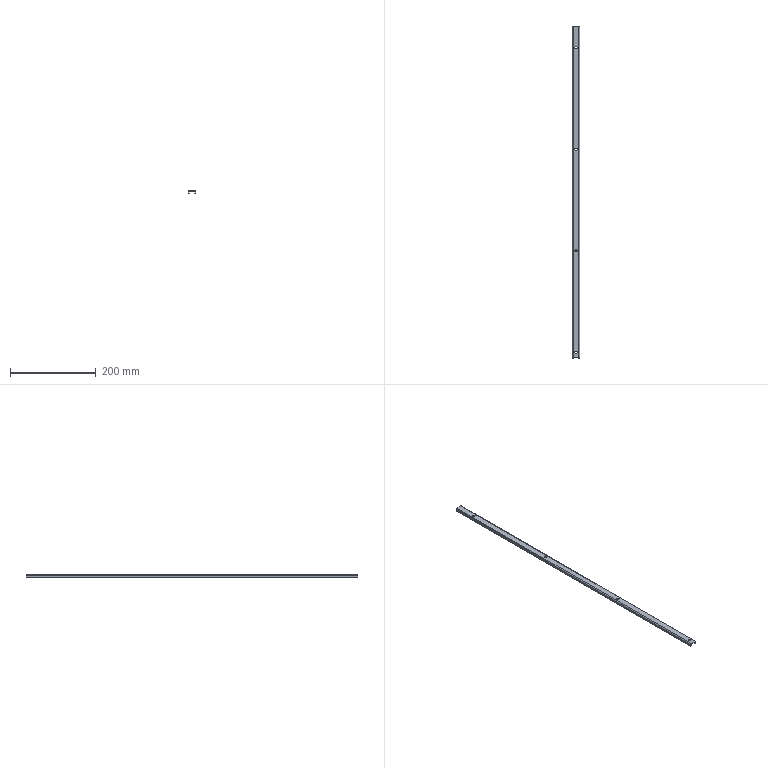Part | NX | features BREP 1 | 1 solid | 40 faces | box 17 x 774.5 x 7 mm | volume 39998 mm3 | plane 22 | cone 8 | cylinder 6 | torus 4 | commonest cylinder face diameters 0.2 x2 2 x2 4.2 x2
STEP:
#1=CARTESIAN_POINT('',(-2.7,336.75,2.));
#2=VERTEX_POINT('',#1);
#3=CARTESIAN_POINT('',(2.7,336.75,2.));
#4=VERTEX_POINT('',#3);
#5=CARTESIAN_POINT('',(0.,336.75,2.));
#6=DIRECTION('',(0.,0.,1.));
#7=DIRECTION('',(1.,0.,0.));
#8=AXIS2_PLACEMENT_3D('',#5,#6,#7);
#9=CIRCLE('',#8,2.7);
#10=EDGE_CURVE('',#2,#4,#9,.T.);
#11=ORIENTED_EDGE('',*,*,#10,.T.);
#12=CARTESIAN_POINT('',(4.7,336.75,0.));
#13=VERTEX_POINT('',#12);
#14=CARTESIAN_POINT('',(4.7,336.75,0.));
#15=DIRECTION('',(0.7071,0.,-0.7071));
#16=VECTOR('',#15,1000.);
#17=LINE('',#14,#16);
#18=EDGE_CURVE('',#4,#13,#17,.T.);
#19=ORIENTED_EDGE('',*,*,#18,.T.);
#20=CARTESIAN_POINT('',(-4.7,336.75,0.));
#21=VERTEX_POINT('',#20);
#22=CARTESIAN_POINT('',(0.,336.75,0.));
#23=DIRECTION('',(0.,0.,-1.));
#24=DIRECTION('',(-1.,0.,0.));
#25=AXIS2_PLACEMENT_3D('',#22,#23,#24);
#26=CIRCLE('',#25,4.7);
#27=EDGE_CURVE('',#13,#21,#26,.T.);
#28=ORIENTED_EDGE('',*,*,#27,.T.);
#29=CARTESIAN_POINT('',(-4.7,336.75,0.));
#30=DIRECTION('',(-0.7071,0.,-0.7071));
#31=VECTOR('',#30,1000.);
#32=LINE('',#29,#31);
#33=EDGE_CURVE('',#2,#21,#32,.T.);
#34=ORIENTED_EDGE('',*,*,#33,.F.);
#35=EDGE_LOOP('',(#11,#19,#28,#34));
#36=FACE_BOUND('',#35,.T.);
#37=CARTESIAN_POINT('',(0.,336.75,0.));
#38=DIRECTION('',(0.,0.,-1.));
#39=DIRECTION('',(-1.,0.,0.));
#40=AXIS2_PLACEMENT_3D('',#37,#38,#39);
#41=CONICAL_SURFACE('',#40,4.7,0.7854);
#42=ADVANCED_FACE('',(#36),#41,.F.);
#43=CARTESIAN_POINT('',(-2.7,99.75,2.));
#44=VERTEX_POINT('',#43);
#45=CARTESIAN_POINT('',(2.7,99.75,2.));
#46=VERTEX_POINT('',#45);
#47=CARTESIAN_POINT('',(0.,99.75,2.));
#48=DIRECTION('',(0.,0.,1.));
#49=DIRECTION('',(1.,0.,0.));
#50=AXIS2_PLACEMENT_3D('',#47,#48,#49);
#51=CIRCLE('',#50,2.7);
#52=EDGE_CURVE('',#44,#46,#51,.T.);
#53=ORIENTED_EDGE('',*,*,#52,.T.);
#54=CARTESIAN_POINT('',(4.7,99.75,0.));
#55=VERTEX_POINT('',#54);
#56=CARTESIAN_POINT('',(4.7,99.75,0.));
#57=DIRECTION('',(0.7071,0.,-0.7071));
#58=VECTOR('',#57,1000.);
#59=LINE('',#56,#58);
#60=EDGE_CURVE('',#46,#55,#59,.T.);
#61=ORIENTED_EDGE('',*,*,#60,.T.);
#62=CARTESIAN_POINT('',(-4.7,99.75,0.));
#63=VERTEX_POINT('',#62);
#64=CARTESIAN_POINT('',(0.,99.75,0.));
#65=DIRECTION('',(0.,0.,-1.));
#66=DIRECTION('',(-1.,0.,0.));
#67=AXIS2_PLACEMENT_3D('',#64,#65,#66);
#68=CIRCLE('',#67,4.7);
#69=EDGE_CURVE('',#55,#63,#68,.T.);
#70=ORIENTED_EDGE('',*,*,#69,.T.);
#71=CARTESIAN_POINT('',(-4.7,99.75,0.));
#72=DIRECTION('',(-0.7071,0.,-0.7071));
#73=VECTOR('',#72,1000.);
#74=LINE('',#71,#73);
#75=EDGE_CURVE('',#44,#63,#74,.T.);
#76=ORIENTED_EDGE('',*,*,#75,.F.);
#77=EDGE_LOOP('',(#53,#61,#70,#76));
#78=FACE_BOUND('',#77,.T.);
#79=CARTESIAN_POINT('',(0.,99.75,0.));
#80=DIRECTION('',(0.,0.,-1.));
#81=DIRECTION('',(-1.,0.,0.));
#82=AXIS2_PLACEMENT_3D('',#79,#80,#81);
#83=CONICAL_SURFACE('',#82,4.7,0.7854);
#84=ADVANCED_FACE('',(#78),#83,.F.);
#85=CARTESIAN_POINT('',(-2.7,-137.25,2.));
#86=VERTEX_POINT('',#85);
#87=CARTESIAN_POINT('',(2.7,-137.25,2.));
#88=VERTEX_POINT('',#87);
#89=CARTESIAN_POINT('',(0.,-137.25,2.));
#90=DIRECTION('',(0.,0.,1.));
#91=DIRECTION('',(1.,0.,0.));
#92=AXIS2_PLACEMENT_3D('',#89,#90,#91);
#93=CIRCLE('',#92,2.7);
#94=EDGE_CURVE('',#86,#88,#93,.T.);
#95=ORIENTED_EDGE('',*,*,#94,.T.);
#96=CARTESIAN_POINT('',(4.7,-137.25,0.));
#97=VERTEX_POINT('',#96);
#98=CARTESIAN_POINT('',(4.7,-137.25,0.));
#99=DIRECTION('',(0.7071,0.,-0.7071));
#100=VECTOR('',#99,1000.);
#101=LINE('',#98,#100);
#102=EDGE_CURVE('',#88,#97,#101,.T.);
#103=ORIENTED_EDGE('',*,*,#102,.T.);
#104=CARTESIAN_POINT('',(-4.7,-137.25,0.));
#105=VERTEX_POINT('',#104);
#106=CARTESIAN_POINT('',(0.,-137.25,0.));
#107=DIRECTION('',(0.,0.,-1.));
#108=DIRECTION('',(-1.,0.,0.));
#109=AXIS2_PLACEMENT_3D('',#106,#107,#108);
#110=CIRCLE('',#109,4.7);
#111=EDGE_CURVE('',#97,#105,#110,.T.);
#112=ORIENTED_EDGE('',*,*,#111,.T.);
#113=CARTESIAN_POINT('',(-4.7,-137.25,0.));
#114=DIRECTION('',(-0.7071,0.,-0.7071));
#115=VECTOR('',#114,1000.);
#116=LINE('',#113,#115);
#117=EDGE_CURVE('',#86,#105,#116,.T.);
#118=ORIENTED_EDGE('',*,*,#117,.F.);
#119=EDGE_LOOP('',(#95,#103,#112,#118));
#120=FACE_BOUND('',#119,.T.);
#121=CARTESIAN_POINT('',(0.,-137.25,0.));
#122=DIRECTION('',(0.,0.,-1.));
#123=DIRECTION('',(-1.,0.,0.));
#124=AXIS2_PLACEMENT_3D('',#121,#122,#123);
#125=CONICAL_SURFACE('',#124,4.7,0.7854);
#126=ADVANCED_FACE('',(#120),#125,.F.);
#127=CARTESIAN_POINT('',(-2.7,-374.25,2.));
#128=VERTEX_POINT('',#127);
#129=CARTESIAN_POINT('',(2.7,-374.25,2.));
#130=VERTEX_POINT('',#129);
#131=CARTESIAN_POINT('',(0.,-374.25,2.));
#132=DIRECTION('',(0.,0.,1.));
#133=DIRECTION('',(1.,0.,0.));
#134=AXIS2_PLACEMENT_3D('',#131,#132,#133);
#135=CIRCLE('',#134,2.7);
#136=EDGE_CURVE('',#128,#130,#135,.T.);
#137=ORIENTED_EDGE('',*,*,#136,.T.);
#138=CARTESIAN_POINT('',(4.7,-374.25,0.));
#139=VERTEX_POINT('',#138);
#140=CARTESIAN_POINT('',(4.7,-374.25,0.));
#141=DIRECTION('',(0.7071,0.,-0.7071));
#142=VECTOR('',#141,1000.);
#143=LINE('',#140,#142);
#144=EDGE_CURVE('',#130,#139,#143,.T.);
#145=ORIENTED_EDGE('',*,*,#144,.T.);
#146=CARTESIAN_POINT('',(-4.7,-374.25,0.));
#147=VERTEX_POINT('',#146);
#148=CARTESIAN_POINT('',(0.,-374.25,0.));
#149=DIRECTION('',(0.,0.,-1.));
#150=DIRECTION('',(-1.,0.,0.));
#151=AXIS2_PLACEMENT_3D('',#148,#149,#150);
#152=CIRCLE('',#151,4.7);
#153=EDGE_CURVE('',#139,#147,#152,.T.);
#154=ORIENTED_EDGE('',*,*,#153,.T.);
#155=CARTESIAN_POINT('',(-4.7,-374.25,0.));
#156=DIRECTION('',(-0.7071,0.,-0.7071));
#157=VECTOR('',#156,1000.);
#158=LINE('',#155,#157);
#159=EDGE_CURVE('',#128,#147,#158,.T.);
#160=ORIENTED_EDGE('',*,*,#159,.F.);
#161=EDGE_LOOP('',(#137,#145,#154,#160));
#162=FACE_BOUND('',#161,.T.);
#163=CARTESIAN_POINT('',(0.,-374.25,0.));
#164=DIRECTION('',(0.,0.,-1.));
#165=DIRECTION('',(-1.,0.,0.));
#166=AXIS2_PLACEMENT_3D('',#163,#164,#165);
#167=CONICAL_SURFACE('',#166,4.7,0.7854);
#168=ADVANCED_FACE('',(#162),#167,.F.);
#169=CARTESIAN_POINT('',(-6.4,386.25,0.));
#170=VERTEX_POINT('',#169);
#171=CARTESIAN_POINT('',(-6.4,-386.25,0.));
#172=VERTEX_POINT('',#171);
#173=CARTESIAN_POINT('',(-6.4,387.25,0.));
#174=DIRECTION('',(0.,-1.,0.));
#175=VECTOR('',#174,1000.);
#176=LINE('',#173,#175);
#177=EDGE_CURVE('',#170,#172,#176,.T.);
#178=ORIENTED_EDGE('',*,*,#177,.F.);
#179=CARTESIAN_POINT('',(6.4,386.25,0.));
#180=VERTEX_POINT('',#179);
#181=CARTESIAN_POINT('',(6.4,386.25,0.));
#182=DIRECTION('',(1.,0.,0.));
#183=VECTOR('',#182,1000.);
#184=LINE('',#181,#183);
#185=EDGE_CURVE('',#170,#180,#184,.T.);
#186=ORIENTED_EDGE('',*,*,#185,.T.);
#187=CARTESIAN_POINT('',(6.4,-386.25,0.));
#188=VERTEX_POINT('',#187);
#189=CARTESIAN_POINT('',(6.4,387.25,0.));
#190=DIRECTION('',(0.,-1.,0.));
#191=VECTOR('',#190,1000.);
#192=LINE('',#189,#191);
#193=EDGE_CURVE('',#180,#188,#192,.T.);
#194=ORIENTED_EDGE('',*,*,#193,.T.);
#195=CARTESIAN_POINT('',(-6.4,-386.25,0.));
#196=DIRECTION('',(-1.,0.,0.));
#197=VECTOR('',#196,1000.);
#198=LINE('',#195,#197);
#199=EDGE_CURVE('',#188,#172,#198,.T.);
#200=ORIENTED_EDGE('',*,*,#199,.T.);
#201=EDGE_LOOP('',(#178,#186,#194,#200));
#202=FACE_BOUND('',#201,.T.);
#203=CARTESIAN_POINT('',(0.,336.75,0.));
#204=DIRECTION('',(0.,0.,-1.));
#205=DIRECTION('',(-1.,0.,0.));
#206=AXIS2_PLACEMENT_3D('',#203,#204,#205);
#207=CIRCLE('',#206,4.7);
#208=EDGE_CURVE('',#21,#13,#207,.T.);
#209=ORIENTED_EDGE('',*,*,#208,.F.);
#210=ORIENTED_EDGE('',*,*,#27,.F.);
#211=EDGE_LOOP('',(#209,#210));
#212=FACE_BOUND('',#211,.T.);
#213=CARTESIAN_POINT('',(0.,99.75,0.));
#214=DIRECTION('',(0.,0.,-1.));
#215=DIRECTION('',(-1.,0.,0.));
#216=AXIS2_PLACEMENT_3D('',#213,#214,#215);
#217=CIRCLE('',#216,4.7);
#218=EDGE_CURVE('',#63,#55,#217,.T.);
#219=ORIENTED_EDGE('',*,*,#218,.F.);
#220=ORIENTED_EDGE('',*,*,#69,.F.);
#221=EDGE_LOOP('',(#219,#220));
#222=FACE_BOUND('',#221,.T.);
#223=CARTESIAN_POINT('',(0.,-374.25,0.));
#224=DIRECTION('',(0.,0.,-1.));
#225=DIRECTION('',(-1.,0.,0.));
#226=AXIS2_PLACEMENT_3D('',#223,#224,#225);
#227=CIRCLE('',#226,4.7);
#228=EDGE_CURVE('',#147,#139,#227,.T.);
#229=ORIENTED_EDGE('',*,*,#228,.F.);
#230=ORIENTED_EDGE('',*,*,#153,.F.);
#231=EDGE_LOOP('',(#229,#230));
#232=FACE_BOUND('',#231,.T.);
#233=CARTESIAN_POINT('',(0.,-137.25,0.));
#234=DIRECTION('',(0.,0.,-1.));
#235=DIRECTION('',(-1.,0.,0.));
#236=AXIS2_PLACEMENT_3D('',#233,#234,#235);
#237=CIRCLE('',#236,4.7);
#238=EDGE_CURVE('',#105,#97,#237,.T.);
#239=ORIENTED_EDGE('',*,*,#238,.F.);
#240=ORIENTED_EDGE('',*,*,#111,.F.);
#241=EDGE_LOOP('',(#239,#240));
#242=FACE_BOUND('',#241,.T.);
#243=CARTESIAN_POINT('',(-6.5,387.25,0.));
#244=DIRECTION('',(0.,0.,1.));
#245=DIRECTION('',(1.,0.,0.));
#246=AXIS2_PLACEMENT_3D('',#243,#244,#245);
#247=PLANE('',#246);
#248=ADVANCED_FACE('',(#202,#212,#222,#232,#242),#247,.F.);
#249=CARTESIAN_POINT('',(6.4,-387.25,2.));
#250=VERTEX_POINT('',#249);
#251=CARTESIAN_POINT('',(-6.4,-387.25,2.));
#252=VERTEX_POINT('',#251);
#253=CARTESIAN_POINT('',(-6.5,-387.25,2.));
#254=DIRECTION('',(-1.,0.,0.));
#255=VECTOR('',#254,1000.);
#256=LINE('',#253,#255);
#257=EDGE_CURVE('',#250,#252,#256,.T.);
#258=ORIENTED_EDGE('',*,*,#257,.F.);
#259=CARTESIAN_POINT('',(6.4,387.25,2.));
#260=VERTEX_POINT('',#259);
#261=CARTESIAN_POINT('',(6.4,387.25,2.));
#262=DIRECTION('',(0.,-1.,0.));
#263=VECTOR('',#262,1000.);
#264=LINE('',#261,#263);
#265=EDGE_CURVE('',#260,#250,#264,.T.);
#266=ORIENTED_EDGE('',*,*,#265,.F.);
#267=CARTESIAN_POINT('',(-6.4,387.25,2.));
#268=VERTEX_POINT('',#267);
#269=CARTESIAN_POINT('',(-6.5,387.25,2.));
#270=DIRECTION('',(-1.,0.,0.));
#271=VECTOR('',#270,1000.);
#272=LINE('',#269,#271);
#273=EDGE_CURVE('',#260,#268,#272,.T.);
#274=ORIENTED_EDGE('',*,*,#273,.T.);
#275=CARTESIAN_POINT('',(-6.4,387.25,2.));
#276=DIRECTION('',(0.,-1.,0.));
#277=VECTOR('',#276,1000.);
#278=LINE('',#275,#277);
#279=EDGE_CURVE('',#268,#252,#278,.T.);
#280=ORIENTED_EDGE('',*,*,#279,.T.);
#281=EDGE_LOOP('',(#258,#266,#274,#280));
#282=FACE_BOUND('',#281,.T.);
#283=ORIENTED_EDGE('',*,*,#10,.F.);
#284=CARTESIAN_POINT('',(0.,336.75,2.));
#285=DIRECTION('',(0.,0.,1.));
#286=DIRECTION('',(1.,0.,0.));
#287=AXIS2_PLACEMENT_3D('',#284,#285,#286);
#288=CIRCLE('',#287,2.7);
#289=EDGE_CURVE('',#4,#2,#288,.T.);
#290=ORIENTED_EDGE('',*,*,#289,.F.);
#291=EDGE_LOOP('',(#283,#290));
#292=FACE_BOUND('',#291,.T.);
#293=ORIENTED_EDGE('',*,*,#52,.F.);
#294=CARTESIAN_POINT('',(0.,99.75,2.));
#295=DIRECTION('',(0.,0.,1.));
#296=DIRECTION('',(1.,0.,0.));
#297=AXIS2_PLACEMENT_3D('',#294,#295,#296);
#298=CIRCLE('',#297,2.7);
#299=EDGE_CURVE('',#46,#44,#298,.T.);
#300=ORIENTED_EDGE('',*,*,#299,.F.);
#301=EDGE_LOOP('',(#293,#300));
#302=FACE_BOUND('',#301,.T.);
#303=ORIENTED_EDGE('',*,*,#94,.F.);
#304=CARTESIAN_POINT('',(0.,-137.25,2.));
#305=DIRECTION('',(0.,0.,1.));
#306=DIRECTION('',(1.,0.,0.));
#307=AXIS2_PLACEMENT_3D('',#304,#305,#306);
#308=CIRCLE('',#307,2.7);
#309=EDGE_CURVE('',#88,#86,#308,.T.);
#310=ORIENTED_EDGE('',*,*,#309,.F.);
#311=EDGE_LOOP('',(#303,#310));
#312=FACE_BOUND('',#311,.T.);
#313=ORIENTED_EDGE('',*,*,#136,.F.);
#314=CARTESIAN_POINT('',(0.,-374.25,2.));
#315=DIRECTION('',(0.,0.,1.));
#316=DIRECTION('',(1.,0.,0.));
#317=AXIS2_PLACEMENT_3D('',#314,#315,#316);
#318=CIRCLE('',#317,2.7);
#319=EDGE_CURVE('',#130,#128,#318,.T.);
#320=ORIENTED_EDGE('',*,*,#319,.F.);
#321=EDGE_LOOP('',(#313,#320));
#322=FACE_BOUND('',#321,.T.);
#323=CARTESIAN_POINT('',(-6.5,387.25,2.));
#324=DIRECTION('',(0.,0.,1.));
#325=DIRECTION('',(1.,0.,0.));
#326=AXIS2_PLACEMENT_3D('',#323,#324,#325);
#327=PLANE('',#326);
#328=ADVANCED_FACE('',(#282,#292,#302,#312,#322),#327,.T.);
#329=CARTESIAN_POINT('',(7.5,387.25,-0.1));
#330=VERTEX_POINT('',#329);
#331=CARTESIAN_POINT('',(8.5,387.25,-0.1));
#332=VERTEX_POINT('',#331);
#333=CARTESIAN_POINT('',(6.5,387.25,-0.1));
#334=DIRECTION('',(1.,0.,0.));
#335=VECTOR('',#334,1000.);
#336=LINE('',#333,#335);
#337=EDGE_CURVE('',#330,#332,#336,.T.);
#338=ORIENTED_EDGE('',*,*,#337,.F.);
#339=CARTESIAN_POINT('',(6.4,387.25,1.));
#340=VERTEX_POINT('',#339);
#341=CARTESIAN_POINT('',(6.4,387.25,-0.1));
#342=DIRECTION('',(0.,-1.,0.));
#343=DIRECTION('',(0.,0.,1.));
#344=AXIS2_PLACEMENT_3D('',#341,#342,#343);
#345=CIRCLE('',#344,1.1);
#346=EDGE_CURVE('',#330,#340,#345,.T.);
#347=ORIENTED_EDGE('',*,*,#346,.T.);
#348=CARTESIAN_POINT('',(6.4,387.25,2.));
#349=DIRECTION('',(0.,0.,-1.));
#350=VECTOR('',#349,1000.);
#351=LINE('',#348,#350);
#352=EDGE_CURVE('',#260,#340,#351,.T.);
#353=ORIENTED_EDGE('',*,*,#352,.F.);
#354=CARTESIAN_POINT('',(6.4,387.25,-0.1));
#355=DIRECTION('',(0.,-1.,0.));
#356=DIRECTION('',(1.,0.,0.));
#357=AXIS2_PLACEMENT_3D('',#354,#355,#356);
#358=CIRCLE('',#357,2.1);
#359=EDGE_CURVE('',#332,#260,#358,.T.);
#360=ORIENTED_EDGE('',*,*,#359,.F.);
#361=EDGE_LOOP('',(#338,#347,#353,#360));
#362=FACE_BOUND('',#361,.T.);
#363=CARTESIAN_POINT('',(6.5,387.25,-0.1));
#364=DIRECTION('',(0.,1.,0.));
#365=DIRECTION('',(1.,0.,0.));
#366=AXIS2_PLACEMENT_3D('',#363,#364,#365);
#367=PLANE('',#366);
#368=ADVANCED_FACE('',(#362),#367,.T.);
#369=CARTESIAN_POINT('',(8.5,387.25,-4.));
#370=VERTEX_POINT('',#369);
#371=CARTESIAN_POINT('',(8.5,387.25,0.));
#372=DIRECTION('',(0.,0.,1.));
#373=VECTOR('',#372,1000.);
#374=LINE('',#371,#373);
#375=EDGE_CURVE('',#370,#332,#374,.T.);
#376=ORIENTED_EDGE('',*,*,#375,.F.);
#377=CARTESIAN_POINT('',(6.5,387.25,-4.));
#378=VERTEX_POINT('',#377);
#379=CARTESIAN_POINT('',(6.4,387.25,-4.));
#380=DIRECTION('',(-1.,0.,0.));
#381=VECTOR('',#380,1000.);
#382=LINE('',#379,#381);
#383=EDGE_CURVE('',#370,#378,#382,.T.);
#384=ORIENTED_EDGE('',*,*,#383,.T.);
#385=CARTESIAN_POINT('',(6.5,387.25,-1.195));
#386=VERTEX_POINT('',#385);
#387=CARTESIAN_POINT('',(6.5,387.25,0.));
#388=DIRECTION('',(0.,0.,1.));
#389=VECTOR('',#388,1000.);
#390=LINE('',#387,#389);
#391=EDGE_CURVE('',#378,#386,#390,.T.);
#392=ORIENTED_EDGE('',*,*,#391,.T.);
#393=CARTESIAN_POINT('',(6.4,387.25,-0.1));
#394=DIRECTION('',(0.,-1.,0.));
#395=DIRECTION('',(0.,0.,1.));
#396=AXIS2_PLACEMENT_3D('',#393,#394,#395);
#397=CIRCLE('',#396,1.1);
#398=EDGE_CURVE('',#386,#330,#397,.T.);
#399=ORIENTED_EDGE('',*,*,#398,.T.);
#400=ORIENTED_EDGE('',*,*,#337,.T.);
#401=EDGE_LOOP('',(#376,#384,#392,#399,#400));
#402=FACE_BOUND('',#401,.T.);
#403=CARTESIAN_POINT('',(6.4,387.25,2.));
#404=DIRECTION('',(0.,1.,0.));
#405=DIRECTION('',(1.,0.,0.));
#406=AXIS2_PLACEMENT_3D('',#403,#404,#405);
#407=PLANE('',#406);
#408=ADVANCED_FACE('',(#402),#407,.T.);
#409=CARTESIAN_POINT('',(6.4,-387.25,1.));
#410=VERTEX_POINT('',#409);
#411=CARTESIAN_POINT('',(6.4,-387.25,0.));
#412=DIRECTION('',(0.,0.,1.));
#413=VECTOR('',#412,1000.);
#414=LINE('',#411,#413);
#415=EDGE_CURVE('',#410,#250,#414,.T.);
#416=ORIENTED_EDGE('',*,*,#415,.F.);
#417=CARTESIAN_POINT('',(7.5,-387.25,-0.1));
#418=VERTEX_POINT('',#417);
#419=CARTESIAN_POINT('',(6.4,-387.25,-0.1));
#420=DIRECTION('',(0.,1.,0.));
#421=DIRECTION('',(0.,0.,-1.));
#422=AXIS2_PLACEMENT_3D('',#419,#420,#421);
#423=CIRCLE('',#422,1.1);
#424=EDGE_CURVE('',#410,#418,#423,.T.);
#425=ORIENTED_EDGE('',*,*,#424,.T.);
#426=CARTESIAN_POINT('',(8.5,-387.25,-0.1));
#427=VERTEX_POINT('',#426);
#428=CARTESIAN_POINT('',(8.5,-387.25,-0.1));
#429=DIRECTION('',(-1.,0.,0.));
#430=VECTOR('',#429,1000.);
#431=LINE('',#428,#430);
#432=EDGE_CURVE('',#427,#418,#431,.T.);
#433=ORIENTED_EDGE('',*,*,#432,.F.);
#434=CARTESIAN_POINT('',(6.4,-387.25,-0.1));
#435=DIRECTION('',(0.,-1.,0.));
#436=DIRECTION('',(1.,0.,0.));
#437=AXIS2_PLACEMENT_3D('',#434,#435,#436);
#438=CIRCLE('',#437,2.1);
#439=EDGE_CURVE('',#427,#250,#438,.T.);
#440=ORIENTED_EDGE('',*,*,#439,.T.);
#441=EDGE_LOOP('',(#416,#425,#433,#440));
#442=FACE_BOUND('',#441,.T.);
#443=CARTESIAN_POINT('',(6.4,-387.25,0.));
#444=DIRECTION('',(0.,-1.,0.));
#445=DIRECTION('',(0.,0.,-1.));
#446=AXIS2_PLACEMENT_3D('',#443,#444,#445);
#447=PLANE('',#446);
#448=ADVANCED_FACE('',(#442),#447,.T.);
#449=CARTESIAN_POINT('',(-6.4,-387.25,1.));
#450=VERTEX_POINT('',#449);
#451=CARTESIAN_POINT('',(-6.4,-387.25,2.));
#452=DIRECTION('',(0.,0.,-1.));
#453=VECTOR('',#452,1000.);
#454=LINE('',#451,#453);
#455=EDGE_CURVE('',#252,#450,#454,.T.);
#456=ORIENTED_EDGE('',*,*,#455,.T.);
#457=CARTESIAN_POINT('',(6.4,-387.25,1.));
#458=DIRECTION('',(1.,0.,0.));
#459=VECTOR('',#458,1000.);
#460=LINE('',#457,#459);
#461=EDGE_CURVE('',#450,#410,#460,.T.);
#462=ORIENTED_EDGE('',*,*,#461,.T.);
#463=ORIENTED_EDGE('',*,*,#415,.T.);
#464=ORIENTED_EDGE('',*,*,#257,.T.);
#465=EDGE_LOOP('',(#456,#462,#463,#464));
#466=FACE_BOUND('',#465,.T.);
#467=CARTESIAN_POINT('',(8.5,-387.25,-0.1));
#468=DIRECTION('',(0.,-1.,0.));
#469=DIRECTION('',(0.,0.,-1.));
#470=AXIS2_PLACEMENT_3D('',#467,#468,#469);
#471=PLANE('',#470);
#472=ADVANCED_FACE('',(#466),#471,.T.);
#473=CARTESIAN_POINT('',(-6.4,387.25,1.));
#474=VERTEX_POINT('',#473);
#475=CARTESIAN_POINT('',(-6.4,387.25,0.));
#476=DIRECTION('',(0.,0.,1.));
#477=VECTOR('',#476,1000.);
#478=LINE('',#475,#477);
#479=EDGE_CURVE('',#474,#268,#478,.T.);
#480=ORIENTED_EDGE('',*,*,#479,.F.);
#481=CARTESIAN_POINT('',(-7.5,387.25,-0.1));
#482=VERTEX_POINT('',#481);
#483=CARTESIAN_POINT('',(-6.4,387.25,-0.1));
#484=DIRECTION('',(0.,-1.,0.));
#485=DIRECTION('',(0.,0.,1.));
#486=AXIS2_PLACEMENT_3D('',#483,#484,#485);
#487=CIRCLE('',#486,1.1);
#488=EDGE_CURVE('',#474,#482,#487,.T.);
#489=ORIENTED_EDGE('',*,*,#488,.T.);
#490=CARTESIAN_POINT('',(-8.5,387.25,-0.1));
#491=VERTEX_POINT('',#490);
#492=CARTESIAN_POINT('',(-8.5,387.25,-0.1));
#493=DIRECTION('',(1.,0.,0.));
#494=VECTOR('',#493,1000.);
#495=LINE('',#492,#494);
#496=EDGE_CURVE('',#491,#482,#495,.T.);
#497=ORIENTED_EDGE('',*,*,#496,.F.);
#498=CARTESIAN_POINT('',(-6.4,387.25,-0.1));
#499=DIRECTION('',(0.,-1.,0.));
#500=DIRECTION('',(1.,0.,0.));
#501=AXIS2_PLACEMENT_3D('',#498,#499,#500);
#502=CIRCLE('',#501,2.1);
#503=EDGE_CURVE('',#268,#491,#502,.T.);
#504=ORIENTED_EDGE('',*,*,#503,.F.);
#505=EDGE_LOOP('',(#480,#489,#497,#504));
#506=FACE_BOUND('',#505,.T.);
#507=CARTESIAN_POINT('',(-6.4,387.25,0.));
#508=DIRECTION('',(0.,1.,0.));
#509=DIRECTION('',(1.,0.,0.));
#510=AXIS2_PLACEMENT_3D('',#507,#508,#509);
#511=PLANE('',#510);
#512=ADVANCED_FACE('',(#506),#511,.T.);
#513=ORIENTED_EDGE('',*,*,#352,.T.);
#514=CARTESIAN_POINT('',(-6.4,387.25,1.));
#515=DIRECTION('',(-1.,0.,0.));
#516=VECTOR('',#515,1000.);
#517=LINE('',#514,#516);
#518=EDGE_CURVE('',#340,#474,#517,.T.);
#519=ORIENTED_EDGE('',*,*,#518,.T.);
#520=ORIENTED_EDGE('',*,*,#479,.T.);
#521=ORIENTED_EDGE('',*,*,#273,.F.);
#522=EDGE_LOOP('',(#513,#519,#520,#521));
#523=FACE_BOUND('',#522,.T.);
#524=CARTESIAN_POINT('',(-8.5,387.25,-0.1));
#525=DIRECTION('',(0.,1.,0.));
#526=DIRECTION('',(1.,0.,0.));
#527=AXIS2_PLACEMENT_3D('',#524,#525,#526);
#528=PLANE('',#527);
#529=ADVANCED_FACE('',(#523),#528,.T.);
#530=CARTESIAN_POINT('',(-7.5,-387.25,-0.1));
#531=VERTEX_POINT('',#530);
#532=CARTESIAN_POINT('',(-8.5,-387.25,-0.1));
#533=VERTEX_POINT('',#532);
#534=CARTESIAN_POINT('',(-6.5,-387.25,-0.1));
#535=DIRECTION('',(-1.,0.,0.));
#536=VECTOR('',#535,1000.);
#537=LINE('',#534,#536);
#538=EDGE_CURVE('',#531,#533,#537,.T.);
#539=ORIENTED_EDGE('',*,*,#538,.F.);
#540=CARTESIAN_POINT('',(-6.4,-387.25,-0.1));
#541=DIRECTION('',(0.,1.,0.));
#542=DIRECTION('',(0.,0.,-1.));
#543=AXIS2_PLACEMENT_3D('',#540,#541,#542);
#544=CIRCLE('',#543,1.1);
#545=EDGE_CURVE('',#531,#450,#544,.T.);
#546=ORIENTED_EDGE('',*,*,#545,.T.);
#547=ORIENTED_EDGE('',*,*,#455,.F.);
#548=CARTESIAN_POINT('',(-6.4,-387.25,-0.1));
#549=DIRECTION('',(0.,-1.,0.));
#550=DIRECTION('',(1.,0.,0.));
#551=AXIS2_PLACEMENT_3D('',#548,#549,#550);
#552=CIRCLE('',#551,2.1);
#553=EDGE_CURVE('',#252,#533,#552,.T.);
#554=ORIENTED_EDGE('',*,*,#553,.T.);
#555=EDGE_LOOP('',(#539,#546,#547,#554));
#556=FACE_BOUND('',#555,.T.);
#557=CARTESIAN_POINT('',(-6.5,-387.25,-0.1));
#558=DIRECTION('',(0.,-1.,0.));
#559=DIRECTION('',(0.,0.,-1.));
#560=AXIS2_PLACEMENT_3D('',#557,#558,#559);
#561=PLANE('',#560);
#562=ADVANCED_FACE('',(#556),#561,.T.);
#563=CARTESIAN_POINT('',(-8.5,-387.25,-4.));
#564=VERTEX_POINT('',#563);
#565=CARTESIAN_POINT('',(-8.5,-387.25,0.));
#566=DIRECTION('',(0.,0.,-1.));
#567=VECTOR('',#566,1000.);
#568=LINE('',#565,#567);
#569=EDGE_CURVE('',#533,#564,#568,.T.);
#570=ORIENTED_EDGE('',*,*,#569,.T.);
#571=CARTESIAN_POINT('',(-6.5,-387.25,-4.));
#572=VERTEX_POINT('',#571);
#573=CARTESIAN_POINT('',(-6.4,-387.25,-4.));
#574=DIRECTION('',(1.,0.,0.));
#575=VECTOR('',#574,1000.);
#576=LINE('',#573,#575);
#577=EDGE_CURVE('',#564,#572,#576,.T.);
#578=ORIENTED_EDGE('',*,*,#577,.T.);
#579=CARTESIAN_POINT('',(-6.5,-387.25,-1.195));
#580=VERTEX_POINT('',#579);
#581=CARTESIAN_POINT('',(-6.5,-387.25,0.));
#582=DIRECTION('',(0.,0.,-1.));
#583=VECTOR('',#582,1000.);
#584=LINE('',#581,#583);
#585=EDGE_CURVE('',#580,#572,#584,.T.);
#586=ORIENTED_EDGE('',*,*,#585,.F.);
#587=CARTESIAN_POINT('',(-6.4,-387.25,-0.1));
#588=DIRECTION('',(0.,1.,0.));
#589=DIRECTION('',(0.,0.,-1.));
#590=AXIS2_PLACEMENT_3D('',#587,#588,#589);
#591=CIRCLE('',#590,1.1);
#592=EDGE_CURVE('',#580,#531,#591,.T.);
#593=ORIENTED_EDGE('',*,*,#592,.T.);
#594=ORIENTED_EDGE('',*,*,#538,.T.);
#595=EDGE_LOOP('',(#570,#578,#586,#593,#594));
#596=FACE_BOUND('',#595,.T.);
#597=CARTESIAN_POINT('',(-6.4,-387.25,2.));
#598=DIRECTION('',(0.,-1.,0.));
#599=DIRECTION('',(0.,0.,-1.));
#600=AXIS2_PLACEMENT_3D('',#597,#598,#599);
#601=PLANE('',#600);
#602=ADVANCED_FACE('',(#596),#601,.T.);
#603=CARTESIAN_POINT('',(-6.5,386.25,-5.));
#604=VERTEX_POINT('',#603);
#605=CARTESIAN_POINT('',(-6.5,-386.25,-5.));
#606=VERTEX_POINT('',#605);
#607=CARTESIAN_POINT('',(-6.5,387.25,-5.));
#608=DIRECTION('',(0.,-1.,0.));
#609=VECTOR('',#608,1000.);
#610=LINE('',#607,#609);
#611=EDGE_CURVE('',#604,#606,#610,.T.);
#612=ORIENTED_EDGE('',*,*,#611,.F.);
#613=CARTESIAN_POINT('',(-6.5,387.25,-4.));
#614=VERTEX_POINT('',#613);
#615=CARTESIAN_POINT('',(-6.5,386.25,-5.));
#616=DIRECTION('',(0.,0.7071,0.7071));
#617=VECTOR('',#616,1000.);
#618=LINE('',#615,#617);
#619=EDGE_CURVE('',#604,#614,#618,.T.);
#620=ORIENTED_EDGE('',*,*,#619,.T.);
#621=CARTESIAN_POINT('',(-6.5,387.25,-1.195));
#622=VERTEX_POINT('',#621);
#623=CARTESIAN_POINT('',(-6.5,387.25,0.));
#624=DIRECTION('',(0.,0.,-1.));
#625=VECTOR('',#624,1000.);
#626=LINE('',#623,#625);
#627=EDGE_CURVE('',#622,#614,#626,.T.);
#628=ORIENTED_EDGE('',*,*,#627,.F.);
#629=CARTESIAN_POINT('',(-6.5,386.25,-0.1));
#630=VERTEX_POINT('',#629);
#631=CARTESIAN_POINT('',(-6.5,387.25,-1.195));
#632=CARTESIAN_POINT('',(-6.5,387.25,-0.9262));
#633=CARTESIAN_POINT('',(-6.5,387.091,-0.5362));
#634=CARTESIAN_POINT('',(-6.5,386.619,-0.219));
#635=CARTESIAN_POINT('',(-6.5,386.413,-0.1517));
#636=CARTESIAN_POINT('',(-6.5,386.25,-0.1));
#637=B_SPLINE_CURVE_WITH_KNOTS('',3,(#631,#632,#633,#634,#635,#636),.UNSPECIFIED.,.F.,.F.,(4,1,1,4),(0.,0.5,0.75,1.),.UNSPECIFIED.);
#638=EDGE_CURVE('',#622,#630,#637,.T.);
#639=ORIENTED_EDGE('',*,*,#638,.T.);
#640=CARTESIAN_POINT('',(-6.5,-386.25,-0.1));
#641=VERTEX_POINT('',#640);
#642=CARTESIAN_POINT('',(-6.5,387.25,-0.1));
#643=DIRECTION('',(0.,-1.,0.));
#644=VECTOR('',#643,1000.);
#645=LINE('',#642,#644);
#646=EDGE_CURVE('',#630,#641,#645,.T.);
#647=ORIENTED_EDGE('',*,*,#646,.T.);
#648=CARTESIAN_POINT('',(-6.5,-386.25,-0.1));
#649=CARTESIAN_POINT('',(-6.5,-386.412,-0.1513));
#650=CARTESIAN_POINT('',(-6.5,-386.619,-0.2191));
#651=CARTESIAN_POINT('',(-6.5,-387.09,-0.5364));
#652=CARTESIAN_POINT('',(-6.5,-387.25,-0.9248));
#653=CARTESIAN_POINT('',(-6.5,-387.25,-1.195));
#654=B_SPLINE_CURVE_WITH_KNOTS('',3,(#648,#649,#650,#651,#652,#653),.UNSPECIFIED.,.F.,.F.,(4,1,1,4),(0.,0.25,0.5,1.),.UNSPECIFIED.);
#655=EDGE_CURVE('',#641,#580,#654,.T.);
#656=ORIENTED_EDGE('',*,*,#655,.T.);
#657=ORIENTED_EDGE('',*,*,#585,.T.);
#658=CARTESIAN_POINT('',(-6.5,-387.25,-4.));
#659=DIRECTION('',(0.,0.7071,-0.7071));
#660=VECTOR('',#659,1000.);
#661=LINE('',#658,#660);
#662=EDGE_CURVE('',#572,#606,#661,.T.);
#663=ORIENTED_EDGE('',*,*,#662,.T.);
#664=EDGE_LOOP('',(#612,#620,#628,#639,#647,#656,#657,#663));
#665=FACE_BOUND('',#664,.T.);
#666=CARTESIAN_POINT('',(-6.5,387.25,0.));
#667=DIRECTION('',(-1.,0.,0.));
#668=DIRECTION('',(0.,1.,0.));
#669=AXIS2_PLACEMENT_3D('',#666,#667,#668);
#670=PLANE('',#669);
#671=ADVANCED_FACE('',(#665),#670,.F.);
#672=CARTESIAN_POINT('',(-8.5,386.25,-5.));
#673=VERTEX_POINT('',#672);
#674=CARTESIAN_POINT('',(-8.5,-386.25,-5.));
#675=VERTEX_POINT('',#674);
#676=CARTESIAN_POINT('',(-8.5,387.25,-5.));
#677=DIRECTION('',(0.,-1.,0.));
#678=VECTOR('',#677,1000.);
#679=LINE('',#676,#678);
#680=EDGE_CURVE('',#673,#675,#679,.T.);
#681=ORIENTED_EDGE('',*,*,#680,.F.);
#682=CARTESIAN_POINT('',(-8.5,386.25,-5.));
#683=DIRECTION('',(1.,0.,0.));
#684=VECTOR('',#683,1000.);
#685=LINE('',#682,#684);
#686=EDGE_CURVE('',#673,#604,#685,.T.);
#687=ORIENTED_EDGE('',*,*,#686,.T.);
#688=ORIENTED_EDGE('',*,*,#611,.T.);
#689=CARTESIAN_POINT('',(-8.5,-386.25,-5.));
#690=DIRECTION('',(-1.,0.,0.));
#691=VECTOR('',#690,1000.);
#692=LINE('',#689,#691);
#693=EDGE_CURVE('',#606,#675,#692,.T.);
#694=ORIENTED_EDGE('',*,*,#693,.T.);
#695=EDGE_LOOP('',(#681,#687,#688,#694));
#696=FACE_BOUND('',#695,.T.);
#697=CARTESIAN_POINT('',(-8.5,387.25,-5.));
#698=DIRECTION('',(0.,0.,-1.));
#699=DIRECTION('',(-1.,0.,0.));
#700=AXIS2_PLACEMENT_3D('',#697,#698,#699);
#701=PLANE('',#700);
#702=ADVANCED_FACE('',(#696),#701,.T.);
#703=CARTESIAN_POINT('',(-8.5,387.25,-4.));
#704=VERTEX_POINT('',#703);
#705=CARTESIAN_POINT('',(-8.5,387.25,0.));
#706=DIRECTION('',(0.,0.,-1.));
#707=VECTOR('',#706,1000.);
#708=LINE('',#705,#707);
#709=EDGE_CURVE('',#491,#704,#708,.T.);
#710=ORIENTED_EDGE('',*,*,#709,.T.);
#711=CARTESIAN_POINT('',(-8.5,389.25,-2.));
#712=DIRECTION('',(0.,-0.7071,-0.7071));
#713=VECTOR('',#712,1000.);
#714=LINE('',#711,#713);
#715=EDGE_CURVE('',#704,#673,#714,.T.);
#716=ORIENTED_EDGE('',*,*,#715,.T.);
#717=ORIENTED_EDGE('',*,*,#680,.T.);
#718=CARTESIAN_POINT('',(-8.5,-2.,-389.25));
#719=DIRECTION('',(0.,-0.7071,0.7071));
#720=VECTOR('',#719,1000.);
#721=LINE('',#718,#720);
#722=EDGE_CURVE('',#675,#564,#721,.T.);
#723=ORIENTED_EDGE('',*,*,#722,.T.);
#724=ORIENTED_EDGE('',*,*,#569,.F.);
#725=CARTESIAN_POINT('',(-8.5,387.25,-0.1));
#726=DIRECTION('',(0.,-1.,0.));
#727=VECTOR('',#726,1000.);
#728=LINE('',#725,#727);
#729=EDGE_CURVE('',#491,#533,#728,.T.);
#730=ORIENTED_EDGE('',*,*,#729,.F.);
#731=EDGE_LOOP('',(#710,#716,#717,#723,#724,#730));
#732=FACE_BOUND('',#731,.T.);
#733=CARTESIAN_POINT('',(-8.5,387.25,0.));
#734=DIRECTION('',(-1.,0.,0.));
#735=DIRECTION('',(0.,1.,0.));
#736=AXIS2_PLACEMENT_3D('',#733,#734,#735);
#737=PLANE('',#736);
#738=ADVANCED_FACE('',(#732),#737,.T.);
#739=ORIENTED_EDGE('',*,*,#553,.F.);
#740=ORIENTED_EDGE('',*,*,#279,.F.);
#741=ORIENTED_EDGE('',*,*,#503,.T.);
#742=ORIENTED_EDGE('',*,*,#729,.T.);
#743=EDGE_LOOP('',(#739,#740,#741,#742));
#744=FACE_BOUND('',#743,.T.);
#745=CARTESIAN_POINT('',(-6.4,387.25,-0.1));
#746=DIRECTION('',(0.,-1.,0.));
#747=DIRECTION('',(0.,0.,-1.));
#748=AXIS2_PLACEMENT_3D('',#745,#746,#747);
#749=CYLINDRICAL_SURFACE('',#748,2.1);
#750=ADVANCED_FACE('',(#744),#749,.T.);
#751=ORIENTED_EDGE('',*,*,#439,.F.);
#752=CARTESIAN_POINT('',(8.5,387.25,-0.1));
#753=DIRECTION('',(0.,-1.,0.));
#754=VECTOR('',#753,1000.);
#755=LINE('',#752,#754);
#756=EDGE_CURVE('',#332,#427,#755,.T.);
#757=ORIENTED_EDGE('',*,*,#756,.F.);
#758=ORIENTED_EDGE('',*,*,#359,.T.);
#759=ORIENTED_EDGE('',*,*,#265,.T.);
#760=EDGE_LOOP('',(#751,#757,#758,#759));
#761=FACE_BOUND('',#760,.T.);
#762=CARTESIAN_POINT('',(6.4,387.25,-0.1));
#763=DIRECTION('',(0.,-1.,0.));
#764=DIRECTION('',(0.,0.,-1.));
#765=AXIS2_PLACEMENT_3D('',#762,#763,#764);
#766=CYLINDRICAL_SURFACE('',#765,2.1);
#767=ADVANCED_FACE('',(#761),#766,.T.);
#768=CARTESIAN_POINT('',(8.5,386.25,-5.));
#769=VERTEX_POINT('',#768);
#770=CARTESIAN_POINT('',(8.5,-386.25,-5.));
#771=VERTEX_POINT('',#770);
#772=CARTESIAN_POINT('',(8.5,387.25,-5.));
#773=DIRECTION('',(0.,-1.,0.));
#774=VECTOR('',#773,1000.);
#775=LINE('',#772,#774);
#776=EDGE_CURVE('',#769,#771,#775,.T.);
#777=ORIENTED_EDGE('',*,*,#776,.F.);
#778=CARTESIAN_POINT('',(8.5,389.25,-2.));
#779=DIRECTION('',(0.,0.7071,0.7071));
#780=VECTOR('',#779,1000.);
#781=LINE('',#778,#780);
#782=EDGE_CURVE('',#769,#370,#781,.T.);
#783=ORIENTED_EDGE('',*,*,#782,.T.);
#784=ORIENTED_EDGE('',*,*,#375,.T.);
#785=ORIENTED_EDGE('',*,*,#756,.T.);
#786=CARTESIAN_POINT('',(8.5,-387.25,-4.));
#787=VERTEX_POINT('',#786);
#788=CARTESIAN_POINT('',(8.5,-387.25,0.));
#789=DIRECTION('',(0.,0.,1.));
#790=VECTOR('',#789,1000.);
#791=LINE('',#788,#790);
#792=EDGE_CURVE('',#787,#427,#791,.T.);
#793=ORIENTED_EDGE('',*,*,#792,.F.);
#794=CARTESIAN_POINT('',(8.5,-2.,-389.25));
#795=DIRECTION('',(0.,0.7071,-0.7071));
#796=VECTOR('',#795,1000.);
#797=LINE('',#794,#796);
#798=EDGE_CURVE('',#787,#771,#797,.T.);
#799=ORIENTED_EDGE('',*,*,#798,.T.);
#800=EDGE_LOOP('',(#777,#783,#784,#785,#793,#799));
#801=FACE_BOUND('',#800,.T.);
#802=CARTESIAN_POINT('',(8.5,387.25,0.));
#803=DIRECTION('',(1.,0.,0.));
#804=DIRECTION('',(0.,1.,0.));
#805=AXIS2_PLACEMENT_3D('',#802,#803,#804);
#806=PLANE('',#805);
#807=ADVANCED_FACE('',(#801),#806,.T.);
#808=CARTESIAN_POINT('',(6.5,386.25,-5.));
#809=VERTEX_POINT('',#808);
#810=CARTESIAN_POINT('',(6.5,-386.25,-5.));
#811=VERTEX_POINT('',#810);
#812=CARTESIAN_POINT('',(6.5,387.25,-5.));
#813=DIRECTION('',(0.,-1.,0.));
#814=VECTOR('',#813,1000.);
#815=LINE('',#812,#814);
#816=EDGE_CURVE('',#809,#811,#815,.T.);
#817=ORIENTED_EDGE('',*,*,#816,.F.);
#818=CARTESIAN_POINT('',(6.5,386.25,-5.));
#819=DIRECTION('',(1.,0.,0.));
#820=VECTOR('',#819,1000.);
#821=LINE('',#818,#820);
#822=EDGE_CURVE('',#809,#769,#821,.T.);
#823=ORIENTED_EDGE('',*,*,#822,.T.);
#824=ORIENTED_EDGE('',*,*,#776,.T.);
#825=CARTESIAN_POINT('',(6.5,-386.25,-5.));
#826=DIRECTION('',(-1.,0.,0.));
#827=VECTOR('',#826,1000.);
#828=LINE('',#825,#827);
#829=EDGE_CURVE('',#771,#811,#828,.T.);
#830=ORIENTED_EDGE('',*,*,#829,.T.);
#831=EDGE_LOOP('',(#817,#823,#824,#830));
#832=FACE_BOUND('',#831,.T.);
#833=CARTESIAN_POINT('',(6.5,387.25,-5.));
#834=DIRECTION('',(0.,0.,-1.));
#835=DIRECTION('',(0.,-1.,0.));
#836=AXIS2_PLACEMENT_3D('',#833,#834,#835);
#837=PLANE('',#836);
#838=ADVANCED_FACE('',(#832),#837,.T.);
#839=ORIENTED_EDGE('',*,*,#391,.F.);
#840=CARTESIAN_POINT('',(6.5,386.25,-5.));
#841=DIRECTION('',(0.,-0.7071,-0.7071));
#842=VECTOR('',#841,1000.);
#843=LINE('',#840,#842);
#844=EDGE_CURVE('',#378,#809,#843,.T.);
#845=ORIENTED_EDGE('',*,*,#844,.T.);
#846=ORIENTED_EDGE('',*,*,#816,.T.);
#847=CARTESIAN_POINT('',(6.5,-387.25,-4.));
#848=VERTEX_POINT('',#847);
#849=CARTESIAN_POINT('',(6.5,-387.25,-4.));
#850=DIRECTION('',(0.,-0.7071,0.7071));
#851=VECTOR('',#850,1000.);
#852=LINE('',#849,#851);
#853=EDGE_CURVE('',#811,#848,#852,.T.);
#854=ORIENTED_EDGE('',*,*,#853,.T.);
#855=CARTESIAN_POINT('',(6.5,-387.25,-1.195));
#856=VERTEX_POINT('',#855);
#857=CARTESIAN_POINT('',(6.5,-387.25,0.));
#858=DIRECTION('',(0.,0.,1.));
#859=VECTOR('',#858,1000.);
#860=LINE('',#857,#859);
#861=EDGE_CURVE('',#848,#856,#860,.T.);
#862=ORIENTED_EDGE('',*,*,#861,.T.);
#863=CARTESIAN_POINT('',(6.5,-386.25,-0.1));
#864=VERTEX_POINT('',#863);
#865=CARTESIAN_POINT('',(6.5,-387.25,-1.195));
#866=CARTESIAN_POINT('',(6.5,-387.25,-0.9262));
#867=CARTESIAN_POINT('',(6.5,-387.091,-0.5362));
#868=CARTESIAN_POINT('',(6.5,-386.619,-0.219));
#869=CARTESIAN_POINT('',(6.5,-386.413,-0.1517));
#870=CARTESIAN_POINT('',(6.5,-386.25,-0.1));
#871=B_SPLINE_CURVE_WITH_KNOTS('',3,(#865,#866,#867,#868,#869,#870),.UNSPECIFIED.,.F.,.F.,(4,1,1,4),(0.,0.5,0.75,1.),.UNSPECIFIED.);
#872=EDGE_CURVE('',#856,#864,#871,.T.);
#873=ORIENTED_EDGE('',*,*,#872,.T.);
#874=CARTESIAN_POINT('',(6.5,386.25,-0.1));
#875=VERTEX_POINT('',#874);
#876=CARTESIAN_POINT('',(6.5,387.25,-0.1));
#877=DIRECTION('',(0.,-1.,0.));
#878=VECTOR('',#877,1000.);
#879=LINE('',#876,#878);
#880=EDGE_CURVE('',#875,#864,#879,.T.);
#881=ORIENTED_EDGE('',*,*,#880,.F.);
#882=CARTESIAN_POINT('',(6.5,386.25,-0.1));
#883=CARTESIAN_POINT('',(6.5,386.412,-0.1513));
#884=CARTESIAN_POINT('',(6.5,386.619,-0.2191));
#885=CARTESIAN_POINT('',(6.5,387.09,-0.5364));
#886=CARTESIAN_POINT('',(6.5,387.25,-0.9248));
#887=CARTESIAN_POINT('',(6.5,387.25,-1.195));
#888=B_SPLINE_CURVE_WITH_KNOTS('',3,(#882,#883,#884,#885,#886,#887),.UNSPECIFIED.,.F.,.F.,(4,1,1,4),(0.,0.25,0.5,1.),.UNSPECIFIED.);
#889=EDGE_CURVE('',#875,#386,#888,.T.);
#890=ORIENTED_EDGE('',*,*,#889,.T.);
#891=EDGE_LOOP('',(#839,#845,#846,#854,#862,#873,#881,#890));
#892=FACE_BOUND('',#891,.T.);
#893=CARTESIAN_POINT('',(6.5,387.25,0.));
#894=DIRECTION('',(1.,0.,0.));
#895=DIRECTION('',(0.,1.,0.));
#896=AXIS2_PLACEMENT_3D('',#893,#894,#895);
#897=PLANE('',#896);
#898=ADVANCED_FACE('',(#892),#897,.F.);
#899=ORIENTED_EDGE('',*,*,#193,.F.);
#900=CARTESIAN_POINT('',(6.4,386.25,-0.1));
#901=DIRECTION('',(0.,1.,0.));
#902=DIRECTION('',(0.,0.,1.));
#903=AXIS2_PLACEMENT_3D('',#900,#901,#902);
#904=CIRCLE('',#903,0.1);
#905=EDGE_CURVE('',#180,#875,#904,.T.);
#906=ORIENTED_EDGE('',*,*,#905,.T.);
#907=ORIENTED_EDGE('',*,*,#880,.T.);
#908=CARTESIAN_POINT('',(6.4,-386.25,-0.1));
#909=DIRECTION('',(0.,-1.,0.));
#910=DIRECTION('',(0.,0.,-1.));
#911=AXIS2_PLACEMENT_3D('',#908,#909,#910);
#912=CIRCLE('',#911,0.1);
#913=EDGE_CURVE('',#864,#188,#912,.T.);
#914=ORIENTED_EDGE('',*,*,#913,.T.);
#915=EDGE_LOOP('',(#899,#906,#907,#914));
#916=FACE_BOUND('',#915,.T.);
#917=CARTESIAN_POINT('',(6.4,387.25,-0.1));
#918=DIRECTION('',(0.,-1.,0.));
#919=DIRECTION('',(0.,0.,-1.));
#920=AXIS2_PLACEMENT_3D('',#917,#918,#919);
#921=CYLINDRICAL_SURFACE('',#920,0.1);
#922=ADVANCED_FACE('',(#916),#921,.F.);
#923=ORIENTED_EDGE('',*,*,#646,.F.);
#924=CARTESIAN_POINT('',(-6.4,386.25,-0.1));
#925=DIRECTION('',(0.,1.,0.));
#926=DIRECTION('',(0.,0.,1.));
#927=AXIS2_PLACEMENT_3D('',#924,#925,#926);
#928=CIRCLE('',#927,0.1);
#929=EDGE_CURVE('',#630,#170,#928,.T.);
#930=ORIENTED_EDGE('',*,*,#929,.T.);
#931=ORIENTED_EDGE('',*,*,#177,.T.);
#932=CARTESIAN_POINT('',(-6.4,-386.25,-0.1));
#933=DIRECTION('',(0.,-1.,0.));
#934=DIRECTION('',(0.,0.,-1.));
#935=AXIS2_PLACEMENT_3D('',#932,#933,#934);
#936=CIRCLE('',#935,0.1);
#937=EDGE_CURVE('',#172,#641,#936,.T.);
#938=ORIENTED_EDGE('',*,*,#937,.T.);
#939=EDGE_LOOP('',(#923,#930,#931,#938));
#940=FACE_BOUND('',#939,.T.);
#941=CARTESIAN_POINT('',(-6.4,387.25,-0.1));
#942=DIRECTION('',(0.,-1.,0.));
#943=DIRECTION('',(0.,0.,-1.));
#944=AXIS2_PLACEMENT_3D('',#941,#942,#943);
#945=CYLINDRICAL_SURFACE('',#944,0.1);
#946=ADVANCED_FACE('',(#940),#945,.F.);
#947=ORIENTED_EDGE('',*,*,#627,.T.);
#948=CARTESIAN_POINT('',(-6.4,387.25,-4.));
#949=DIRECTION('',(-1.,0.,0.));
#950=VECTOR('',#949,1000.);
#951=LINE('',#948,#950);
#952=EDGE_CURVE('',#614,#704,#951,.T.);
#953=ORIENTED_EDGE('',*,*,#952,.T.);
#954=ORIENTED_EDGE('',*,*,#709,.F.);
#955=ORIENTED_EDGE('',*,*,#496,.T.);
#956=CARTESIAN_POINT('',(-6.4,387.25,-0.1));
#957=DIRECTION('',(0.,-1.,0.));
#958=DIRECTION('',(0.,0.,1.));
#959=AXIS2_PLACEMENT_3D('',#956,#957,#958);
#960=CIRCLE('',#959,1.1);
#961=EDGE_CURVE('',#482,#622,#960,.T.);
#962=ORIENTED_EDGE('',*,*,#961,.T.);
#963=EDGE_LOOP('',(#947,#953,#954,#955,#962));
#964=FACE_BOUND('',#963,.T.);
#965=CARTESIAN_POINT('',(-6.4,387.25,-0.1));
#966=DIRECTION('',(0.,1.,0.));
#967=DIRECTION('',(1.,0.,0.));
#968=AXIS2_PLACEMENT_3D('',#965,#966,#967);
#969=PLANE('',#968);
#970=ADVANCED_FACE('',(#964),#969,.T.);
#971=ORIENTED_EDGE('',*,*,#861,.F.);
#972=CARTESIAN_POINT('',(8.5,-387.25,-4.));
#973=DIRECTION('',(1.,0.,0.));
#974=VECTOR('',#973,1000.);
#975=LINE('',#972,#974);
#976=EDGE_CURVE('',#848,#787,#975,.T.);
#977=ORIENTED_EDGE('',*,*,#976,.T.);
#978=ORIENTED_EDGE('',*,*,#792,.T.);
#979=ORIENTED_EDGE('',*,*,#432,.T.);
#980=CARTESIAN_POINT('',(6.4,-387.25,-0.1));
#981=DIRECTION('',(0.,1.,0.));
#982=DIRECTION('',(0.,0.,-1.));
#983=AXIS2_PLACEMENT_3D('',#980,#981,#982);
#984=CIRCLE('',#983,1.1);
#985=EDGE_CURVE('',#418,#856,#984,.T.);
#986=ORIENTED_EDGE('',*,*,#985,.T.);
#987=EDGE_LOOP('',(#971,#977,#978,#979,#986));
#988=FACE_BOUND('',#987,.T.);
#989=CARTESIAN_POINT('',(-6.4,-387.25,-0.1));
#990=DIRECTION('',(0.,1.,0.));
#991=DIRECTION('',(1.,0.,0.));
#992=AXIS2_PLACEMENT_3D('',#989,#990,#991);
#993=PLANE('',#992);
#994=ADVANCED_FACE('',(#988),#993,.F.);
#995=ORIENTED_EDGE('',*,*,#144,.F.);
#996=ORIENTED_EDGE('',*,*,#319,.T.);
#997=ORIENTED_EDGE('',*,*,#159,.T.);
#998=ORIENTED_EDGE('',*,*,#228,.T.);
#999=EDGE_LOOP('',(#995,#996,#997,#998));
#1000=FACE_BOUND('',#999,.T.);
#1001=CARTESIAN_POINT('',(0.,-374.25,0.));
#1002=DIRECTION('',(0.,0.,-1.));
#1003=DIRECTION('',(-1.,0.,0.));
#1004=AXIS2_PLACEMENT_3D('',#1001,#1002,#1003);
#1005=CONICAL_SURFACE('',#1004,4.7,0.7854);
#1006=ADVANCED_FACE('',(#1000),#1005,.F.);
#1007=ORIENTED_EDGE('',*,*,#102,.F.);
#1008=ORIENTED_EDGE('',*,*,#309,.T.);
#1009=ORIENTED_EDGE('',*,*,#117,.T.);
#1010=ORIENTED_EDGE('',*,*,#238,.T.);
#1011=EDGE_LOOP('',(#1007,#1008,#1009,#1010));
#1012=FACE_BOUND('',#1011,.T.);
#1013=CARTESIAN_POINT('',(0.,-137.25,0.));
#1014=DIRECTION('',(0.,0.,-1.));
#1015=DIRECTION('',(-1.,0.,0.));
#1016=AXIS2_PLACEMENT_3D('',#1013,#1014,#1015);
#1017=CONICAL_SURFACE('',#1016,4.7,0.7854);
#1018=ADVANCED_FACE('',(#1012),#1017,.F.);
#1019=ORIENTED_EDGE('',*,*,#60,.F.);
#1020=ORIENTED_EDGE('',*,*,#299,.T.);
#1021=ORIENTED_EDGE('',*,*,#75,.T.);
#1022=ORIENTED_EDGE('',*,*,#218,.T.);
#1023=EDGE_LOOP('',(#1019,#1020,#1021,#1022));
#1024=FACE_BOUND('',#1023,.T.);
#1025=CARTESIAN_POINT('',(0.,99.75,0.));
#1026=DIRECTION('',(0.,0.,-1.));
#1027=DIRECTION('',(-1.,0.,0.));
#1028=AXIS2_PLACEMENT_3D('',#1025,#1026,#1027);
#1029=CONICAL_SURFACE('',#1028,4.7,0.7854);
#1030=ADVANCED_FACE('',(#1024),#1029,.F.);
#1031=ORIENTED_EDGE('',*,*,#18,.F.);
#1032=ORIENTED_EDGE('',*,*,#289,.T.);
#1033=ORIENTED_EDGE('',*,*,#33,.T.);
#1034=ORIENTED_EDGE('',*,*,#208,.T.);
#1035=EDGE_LOOP('',(#1031,#1032,#1033,#1034));
#1036=FACE_BOUND('',#1035,.T.);
#1037=CARTESIAN_POINT('',(0.,336.75,0.));
#1038=DIRECTION('',(0.,0.,-1.));
#1039=DIRECTION('',(-1.,0.,0.));
#1040=AXIS2_PLACEMENT_3D('',#1037,#1038,#1039);
#1041=CONICAL_SURFACE('',#1040,4.7,0.7854);
#1042=ADVANCED_FACE('',(#1036),#1041,.F.);
#1043=ORIENTED_EDGE('',*,*,#961,.F.);
#1044=ORIENTED_EDGE('',*,*,#488,.F.);
#1045=CARTESIAN_POINT('',(-6.4,386.25,1.));
#1046=DIRECTION('',(1.,0.,0.));
#1047=DIRECTION('',(0.,0.,-1.));
#1048=AXIS2_PLACEMENT_3D('',#1045,#1046,#1047);
#1049=CIRCLE('',#1048,1.);
#1050=EDGE_CURVE('',#170,#474,#1049,.T.);
#1051=ORIENTED_EDGE('',*,*,#1050,.F.);
#1052=ORIENTED_EDGE('',*,*,#929,.F.);
#1053=ORIENTED_EDGE('',*,*,#638,.F.);
#1054=EDGE_LOOP('',(#1043,#1044,#1051,#1052,#1053));
#1055=FACE_BOUND('',#1054,.T.);
#1056=CARTESIAN_POINT('',(-6.4,386.25,-0.1));
#1057=DIRECTION('',(0.,1.,0.));
#1058=DIRECTION('',(0.,0.,1.));
#1059=AXIS2_PLACEMENT_3D('',#1056,#1057,#1058);
#1060=TOROIDAL_SURFACE('',#1059,1.1,1.);
#1061=ADVANCED_FACE('',(#1055),#1060,.T.);
#1062=ORIENTED_EDGE('',*,*,#1050,.T.);
#1063=ORIENTED_EDGE('',*,*,#518,.F.);
#1064=CARTESIAN_POINT('',(6.4,386.25,1.));
#1065=DIRECTION('',(1.,0.,0.));
#1066=DIRECTION('',(0.,0.,-1.));
#1067=AXIS2_PLACEMENT_3D('',#1064,#1065,#1066);
#1068=CIRCLE('',#1067,1.);
#1069=EDGE_CURVE('',#180,#340,#1068,.T.);
#1070=ORIENTED_EDGE('',*,*,#1069,.F.);
#1071=ORIENTED_EDGE('',*,*,#185,.F.);
#1072=EDGE_LOOP('',(#1062,#1063,#1070,#1071));
#1073=FACE_BOUND('',#1072,.T.);
#1074=CARTESIAN_POINT('',(-8.5,386.25,1.));
#1075=DIRECTION('',(1.,0.,0.));
#1076=DIRECTION('',(0.,0.,-1.));
#1077=AXIS2_PLACEMENT_3D('',#1074,#1075,#1076);
#1078=CYLINDRICAL_SURFACE('',#1077,1.);
#1079=ADVANCED_FACE('',(#1073),#1078,.T.);
#1080=ORIENTED_EDGE('',*,*,#889,.F.);
#1081=ORIENTED_EDGE('',*,*,#905,.F.);
#1082=ORIENTED_EDGE('',*,*,#1069,.T.);
#1083=ORIENTED_EDGE('',*,*,#346,.F.);
#1084=ORIENTED_EDGE('',*,*,#398,.F.);
#1085=EDGE_LOOP('',(#1080,#1081,#1082,#1083,#1084));
#1086=FACE_BOUND('',#1085,.T.);
#1087=CARTESIAN_POINT('',(6.4,386.25,-0.1));
#1088=DIRECTION('',(0.,1.,0.));
#1089=DIRECTION('',(0.,0.,1.));
#1090=AXIS2_PLACEMENT_3D('',#1087,#1088,#1089);
#1091=TOROIDAL_SURFACE('',#1090,1.1,1.);
#1092=ADVANCED_FACE('',(#1086),#1091,.T.);
#1093=ORIENTED_EDGE('',*,*,#655,.F.);
#1094=ORIENTED_EDGE('',*,*,#937,.F.);
#1095=CARTESIAN_POINT('',(-6.4,-386.25,1.));
#1096=DIRECTION('',(1.,0.,0.));
#1097=DIRECTION('',(0.,0.,-1.));
#1098=AXIS2_PLACEMENT_3D('',#1095,#1096,#1097);
#1099=CIRCLE('',#1098,1.);
#1100=EDGE_CURVE('',#450,#172,#1099,.T.);
#1101=ORIENTED_EDGE('',*,*,#1100,.F.);
#1102=ORIENTED_EDGE('',*,*,#545,.F.);
#1103=ORIENTED_EDGE('',*,*,#592,.F.);
#1104=EDGE_LOOP('',(#1093,#1094,#1101,#1102,#1103));
#1105=FACE_BOUND('',#1104,.T.);
#1106=CARTESIAN_POINT('',(-6.4,-386.25,-0.1));
#1107=DIRECTION('',(0.,-1.,0.));
#1108=DIRECTION('',(0.,0.,-1.));
#1109=AXIS2_PLACEMENT_3D('',#1106,#1107,#1108);
#1110=TOROIDAL_SURFACE('',#1109,1.1,1.);
#1111=ADVANCED_FACE('',(#1105),#1110,.T.);
#1112=ORIENTED_EDGE('',*,*,#1100,.T.);
#1113=ORIENTED_EDGE('',*,*,#199,.F.);
#1114=CARTESIAN_POINT('',(6.4,-386.25,1.));
#1115=DIRECTION('',(1.,0.,0.));
#1116=DIRECTION('',(0.,0.,-1.));
#1117=AXIS2_PLACEMENT_3D('',#1114,#1115,#1116);
#1118=CIRCLE('',#1117,1.);
#1119=EDGE_CURVE('',#410,#188,#1118,.T.);
#1120=ORIENTED_EDGE('',*,*,#1119,.F.);
#1121=ORIENTED_EDGE('',*,*,#461,.F.);
#1122=EDGE_LOOP('',(#1112,#1113,#1120,#1121));
#1123=FACE_BOUND('',#1122,.T.);
#1124=CARTESIAN_POINT('',(-6.5,-386.25,1.));
#1125=DIRECTION('',(1.,0.,0.));
#1126=DIRECTION('',(0.,0.,-1.));
#1127=AXIS2_PLACEMENT_3D('',#1124,#1125,#1126);
#1128=CYLINDRICAL_SURFACE('',#1127,1.);
#1129=ADVANCED_FACE('',(#1123),#1128,.T.);
#1130=ORIENTED_EDGE('',*,*,#985,.F.);
#1131=ORIENTED_EDGE('',*,*,#424,.F.);
#1132=ORIENTED_EDGE('',*,*,#1119,.T.);
#1133=ORIENTED_EDGE('',*,*,#913,.F.);
#1134=ORIENTED_EDGE('',*,*,#872,.F.);
#1135=EDGE_LOOP('',(#1130,#1131,#1132,#1133,#1134));
#1136=FACE_BOUND('',#1135,.T.);
#1137=CARTESIAN_POINT('',(6.4,-386.25,-0.1));
#1138=DIRECTION('',(0.,-1.,0.));
#1139=DIRECTION('',(0.,0.,-1.));
#1140=AXIS2_PLACEMENT_3D('',#1137,#1138,#1139);
#1141=TOROIDAL_SURFACE('',#1140,1.1,1.);
#1142=ADVANCED_FACE('',(#1136),#1141,.T.);
#1143=ORIENTED_EDGE('',*,*,#715,.F.);
#1144=ORIENTED_EDGE('',*,*,#952,.F.);
#1145=ORIENTED_EDGE('',*,*,#619,.F.);
#1146=ORIENTED_EDGE('',*,*,#686,.F.);
#1147=EDGE_LOOP('',(#1143,#1144,#1145,#1146));
#1148=FACE_BOUND('',#1147,.T.);
#1149=CARTESIAN_POINT('',(-8.5,386.25,-5.));
#1150=DIRECTION('',(0.,-0.7071,0.7071));
#1151=DIRECTION('',(-1.,0.,0.));
#1152=AXIS2_PLACEMENT_3D('',#1149,#1150,#1151);
#1153=PLANE('',#1152);
#1154=ADVANCED_FACE('',(#1148),#1153,.F.);
#1155=ORIENTED_EDGE('',*,*,#844,.F.);
#1156=ORIENTED_EDGE('',*,*,#383,.F.);
#1157=ORIENTED_EDGE('',*,*,#782,.F.);
#1158=ORIENTED_EDGE('',*,*,#822,.F.);
#1159=EDGE_LOOP('',(#1155,#1156,#1157,#1158));
#1160=FACE_BOUND('',#1159,.T.);
#1161=CARTESIAN_POINT('',(6.5,386.25,-5.));
#1162=DIRECTION('',(0.,-0.7071,0.7071));
#1163=DIRECTION('',(-1.,0.,0.));
#1164=AXIS2_PLACEMENT_3D('',#1161,#1162,#1163);
#1165=PLANE('',#1164);
#1166=ADVANCED_FACE('',(#1160),#1165,.F.);
#1167=ORIENTED_EDGE('',*,*,#853,.F.);
#1168=ORIENTED_EDGE('',*,*,#829,.F.);
#1169=ORIENTED_EDGE('',*,*,#798,.F.);
#1170=ORIENTED_EDGE('',*,*,#976,.F.);
#1171=EDGE_LOOP('',(#1167,#1168,#1169,#1170));
#1172=FACE_BOUND('',#1171,.T.);
#1173=CARTESIAN_POINT('',(-6.4,-387.25,-4.));
#1174=DIRECTION('',(0.,-0.7071,-0.7071));
#1175=DIRECTION('',(0.,-0.7071,0.7071));
#1176=AXIS2_PLACEMENT_3D('',#1173,#1174,#1175);
#1177=PLANE('',#1176);
#1178=ADVANCED_FACE('',(#1172),#1177,.T.);
#1179=ORIENTED_EDGE('',*,*,#722,.F.);
#1180=ORIENTED_EDGE('',*,*,#693,.F.);
#1181=ORIENTED_EDGE('',*,*,#662,.F.);
#1182=ORIENTED_EDGE('',*,*,#577,.F.);
#1183=EDGE_LOOP('',(#1179,#1180,#1181,#1182));
#1184=FACE_BOUND('',#1183,.T.);
#1185=CARTESIAN_POINT('',(-6.4,-387.25,-4.));
#1186=DIRECTION('',(0.,0.7071,0.7071));
#1187=DIRECTION('',(1.,0.,0.));
#1188=AXIS2_PLACEMENT_3D('',#1185,#1186,#1187);
#1189=PLANE('',#1188);
#1190=ADVANCED_FACE('',(#1184),#1189,.F.);
#1191=CLOSED_SHELL('',(#42,#84,#126,#168,#248,#328,#368,#408,#448,#472,#512,#529,#562,#602,#671,#702,#738,#750,#767,#807,#838,#898,#922,#946,#970,#994,#1006,#1018,#1030,#1042,#1061,#1079,#1092,#1111,#1129,#1142,#1154,#1166,#1178,#1190));
#1192=MANIFOLD_SOLID_BREP('',#1191);
#1193=(LENGTH_UNIT()NAMED_UNIT(*)SI_UNIT(.MILLI.,.METRE.));
#1194=UNCERTAINTY_MEASURE_WITH_UNIT(LENGTH_MEASURE(0.0508),#1193,'','');
#1195=(NAMED_UNIT(*)PLANE_ANGLE_UNIT()SI_UNIT($,.RADIAN.));
#1196=(NAMED_UNIT(*)SI_UNIT($,.STERADIAN.)SOLID_ANGLE_UNIT());
#1197=(GEOMETRIC_REPRESENTATION_CONTEXT(3)GLOBAL_UNCERTAINTY_ASSIGNED_CONTEXT((#1194))GLOBAL_UNIT_ASSIGNED_CONTEXT((#1193,#1195,#1196))REPRESENTATION_CONTEXT('',''));
#1198=ADVANCED_BREP_SHAPE_REPRESENTATION('',(#1192),#1197);